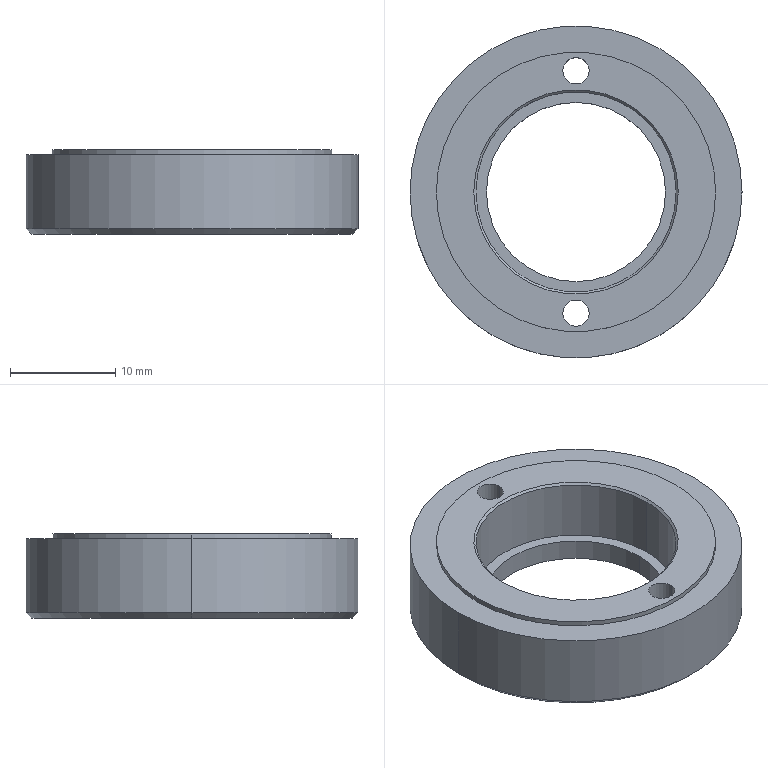Part | SolidWorks | features Chamfer 2, ICE 2, Extrusion 1, HoleWzd 1, MirrorPattern 1 | 1 solid | 20 faces | box 31.5 x 31.5 x 8 mm | volume 3885 mm3 | cylinder 12 | cone 4 | plane 4 | commonest cylinder face diameters 2.5 x4 17 x2 19 x2 26.5 x2 31.5 x2
STEP:
#1=CARTESIAN_POINT('',(-15.25,0.,-4.));
#2=VERTEX_POINT('',#1);
#3=CARTESIAN_POINT('',(15.25,0.,-4.));
#4=VERTEX_POINT('',#3);
#5=CARTESIAN_POINT('',(0.,0.,-4.));
#6=DIRECTION('',(0.,0.,-1.));
#7=DIRECTION('',(1.,0.,0.));
#8=AXIS2_PLACEMENT_3D('',#5,#6,#7);
#9=CIRCLE('',#8,15.25);
#10=EDGE_CURVE('',#2,#4,#9,.T.);
#11=ORIENTED_EDGE('',*,*,#10,.F.);
#12=CARTESIAN_POINT('',(-15.75,0.,-3.5));
#13=VERTEX_POINT('',#12);
#14=CARTESIAN_POINT('',(-15.75,0.,-3.5));
#15=DIRECTION('',(-0.7071,0.,0.7071));
#16=VECTOR('',#15,1000.);
#17=LINE('',#14,#16);
#18=EDGE_CURVE('',#2,#13,#17,.T.);
#19=ORIENTED_EDGE('',*,*,#18,.T.);
#20=CARTESIAN_POINT('',(15.75,0.,-3.5));
#21=VERTEX_POINT('',#20);
#22=CARTESIAN_POINT('',(0.,0.,-3.5));
#23=DIRECTION('',(0.,0.,1.));
#24=DIRECTION('',(1.,0.,0.));
#25=AXIS2_PLACEMENT_3D('',#22,#23,#24);
#26=CIRCLE('',#25,15.75);
#27=EDGE_CURVE('',#21,#13,#26,.T.);
#28=ORIENTED_EDGE('',*,*,#27,.F.);
#29=CARTESIAN_POINT('',(15.75,0.,-3.5));
#30=DIRECTION('',(0.7071,0.,0.7071));
#31=VECTOR('',#30,1000.);
#32=LINE('',#29,#31);
#33=EDGE_CURVE('',#4,#21,#32,.T.);
#34=ORIENTED_EDGE('',*,*,#33,.F.);
#35=EDGE_LOOP('',(#11,#19,#28,#34));
#36=FACE_OUTER_BOUND('',#35,.T.);
#37=CARTESIAN_POINT('',(0.,0.,-3.5));
#38=DIRECTION('',(0.,0.,1.));
#39=DIRECTION('',(1.,0.,0.));
#40=AXIS2_PLACEMENT_3D('',#37,#38,#39);
#41=CONICAL_SURFACE('',#40,15.75,0.7854);
#42=ADVANCED_FACE('',(#36),#41,.T.);
#43=CARTESIAN_POINT('',(13.25,0.,3.55));
#44=VERTEX_POINT('',#43);
#45=CARTESIAN_POINT('',(-13.25,0.,3.55));
#46=VERTEX_POINT('',#45);
#47=CARTESIAN_POINT('',(0.,0.,3.55));
#48=DIRECTION('',(0.,0.,1.));
#49=DIRECTION('',(1.,0.,0.));
#50=AXIS2_PLACEMENT_3D('',#47,#48,#49);
#51=CIRCLE('',#50,13.25);
#52=EDGE_CURVE('',#44,#46,#51,.T.);
#53=ORIENTED_EDGE('',*,*,#52,.T.);
#54=CARTESIAN_POINT('',(-13.25,0.,4.));
#55=VERTEX_POINT('',#54);
#56=CARTESIAN_POINT('',(-13.25,0.,3.55));
#57=DIRECTION('',(0.,0.,1.));
#58=VECTOR('',#57,1000.);
#59=LINE('',#56,#58);
#60=EDGE_CURVE('',#46,#55,#59,.T.);
#61=ORIENTED_EDGE('',*,*,#60,.T.);
#62=CARTESIAN_POINT('',(13.25,0.,4.));
#63=VERTEX_POINT('',#62);
#64=CARTESIAN_POINT('',(0.,0.,4.));
#65=DIRECTION('',(0.,0.,1.));
#66=DIRECTION('',(1.,0.,0.));
#67=AXIS2_PLACEMENT_3D('',#64,#65,#66);
#68=CIRCLE('',#67,13.25);
#69=EDGE_CURVE('',#63,#55,#68,.T.);
#70=ORIENTED_EDGE('',*,*,#69,.F.);
#71=CARTESIAN_POINT('',(13.25,0.,3.55));
#72=DIRECTION('',(0.,0.,1.));
#73=VECTOR('',#72,1000.);
#74=LINE('',#71,#73);
#75=EDGE_CURVE('',#44,#63,#74,.T.);
#76=ORIENTED_EDGE('',*,*,#75,.F.);
#77=EDGE_LOOP('',(#53,#61,#70,#76));
#78=FACE_OUTER_BOUND('',#77,.T.);
#79=CARTESIAN_POINT('',(0.,0.,3.55));
#80=DIRECTION('',(0.,0.,1.));
#81=DIRECTION('',(1.,0.,0.));
#82=AXIS2_PLACEMENT_3D('',#79,#80,#81);
#83=CYLINDRICAL_SURFACE('',#82,13.25);
#84=ADVANCED_FACE('',(#78),#83,.T.);
#85=CARTESIAN_POINT('',(-9.5,0.,3.8));
#86=VERTEX_POINT('',#85);
#87=CARTESIAN_POINT('',(9.5,0.,3.8));
#88=VERTEX_POINT('',#87);
#89=CARTESIAN_POINT('',(0.,0.,3.8));
#90=DIRECTION('',(0.,0.,1.));
#91=DIRECTION('',(1.,0.,0.));
#92=AXIS2_PLACEMENT_3D('',#89,#90,#91);
#93=CIRCLE('',#92,9.5);
#94=EDGE_CURVE('',#86,#88,#93,.T.);
#95=ORIENTED_EDGE('',*,*,#94,.F.);
#96=CARTESIAN_POINT('',(-9.7,0.,4.));
#97=VERTEX_POINT('',#96);
#98=CARTESIAN_POINT('',(-9.5,0.,3.8));
#99=DIRECTION('',(-0.7071,0.,0.7071));
#100=VECTOR('',#99,1000.);
#101=LINE('',#98,#100);
#102=EDGE_CURVE('',#86,#97,#101,.T.);
#103=ORIENTED_EDGE('',*,*,#102,.T.);
#104=CARTESIAN_POINT('',(9.7,0.,4.));
#105=VERTEX_POINT('',#104);
#106=CARTESIAN_POINT('',(0.,0.,4.));
#107=DIRECTION('',(0.,0.,-1.));
#108=DIRECTION('',(1.,0.,0.));
#109=AXIS2_PLACEMENT_3D('',#106,#107,#108);
#110=CIRCLE('',#109,9.7);
#111=EDGE_CURVE('',#105,#97,#110,.T.);
#112=ORIENTED_EDGE('',*,*,#111,.F.);
#113=CARTESIAN_POINT('',(9.5,0.,3.8));
#114=DIRECTION('',(0.7071,0.,0.7071));
#115=VECTOR('',#114,1000.);
#116=LINE('',#113,#115);
#117=EDGE_CURVE('',#88,#105,#116,.T.);
#118=ORIENTED_EDGE('',*,*,#117,.F.);
#119=EDGE_LOOP('',(#95,#103,#112,#118));
#120=FACE_OUTER_BOUND('',#119,.T.);
#121=CARTESIAN_POINT('',(0.,0.,3.8));
#122=DIRECTION('',(0.,0.,1.));
#123=DIRECTION('',(1.,0.,0.));
#124=AXIS2_PLACEMENT_3D('',#121,#122,#123);
#125=CONICAL_SURFACE('',#124,9.5,0.7854);
#126=ADVANCED_FACE('',(#120),#125,.F.);
#127=CARTESIAN_POINT('',(-1.25,11.5,-4.));
#128=VERTEX_POINT('',#127);
#129=CARTESIAN_POINT('',(1.25,11.5,-4.));
#130=VERTEX_POINT('',#129);
#131=CARTESIAN_POINT('',(0.,11.5,-4.));
#132=DIRECTION('',(0.,0.,1.));
#133=DIRECTION('',(1.,0.,0.));
#134=AXIS2_PLACEMENT_3D('',#131,#132,#133);
#135=CIRCLE('',#134,1.25);
#136=EDGE_CURVE('',#128,#130,#135,.T.);
#137=ORIENTED_EDGE('',*,*,#136,.F.);
#138=CARTESIAN_POINT('',(-1.25,11.5,4.));
#139=VERTEX_POINT('',#138);
#140=CARTESIAN_POINT('',(-1.25,11.5,4.));
#141=DIRECTION('',(0.,0.,1.));
#142=VECTOR('',#141,1000.);
#143=LINE('',#140,#142);
#144=EDGE_CURVE('',#128,#139,#143,.T.);
#145=ORIENTED_EDGE('',*,*,#144,.T.);
#146=CARTESIAN_POINT('',(1.25,11.5,4.));
#147=VERTEX_POINT('',#146);
#148=CARTESIAN_POINT('',(0.,11.5,4.));
#149=DIRECTION('',(0.,0.,1.));
#150=DIRECTION('',(1.,0.,0.));
#151=AXIS2_PLACEMENT_3D('',#148,#149,#150);
#152=CIRCLE('',#151,1.25);
#153=EDGE_CURVE('',#139,#147,#152,.T.);
#154=ORIENTED_EDGE('',*,*,#153,.T.);
#155=CARTESIAN_POINT('',(1.25,11.5,4.));
#156=DIRECTION('',(0.,0.,1.));
#157=VECTOR('',#156,1000.);
#158=LINE('',#155,#157);
#159=EDGE_CURVE('',#130,#147,#158,.T.);
#160=ORIENTED_EDGE('',*,*,#159,.F.);
#161=EDGE_LOOP('',(#137,#145,#154,#160));
#162=FACE_OUTER_BOUND('',#161,.T.);
#163=CARTESIAN_POINT('',(0.,11.5,4.));
#164=DIRECTION('',(0.,0.,1.));
#165=DIRECTION('',(1.,0.,0.));
#166=AXIS2_PLACEMENT_3D('',#163,#164,#165);
#167=CYLINDRICAL_SURFACE('',#166,1.25);
#168=ADVANCED_FACE('',(#162),#167,.F.);
#169=CARTESIAN_POINT('',(-1.25,-11.5,-4.));
#170=VERTEX_POINT('',#169);
#171=CARTESIAN_POINT('',(1.25,-11.5,-4.));
#172=VERTEX_POINT('',#171);
#173=CARTESIAN_POINT('',(0.,-11.5,-4.));
#174=DIRECTION('',(0.,0.,1.));
#175=DIRECTION('',(1.,0.,0.));
#176=AXIS2_PLACEMENT_3D('',#173,#174,#175);
#177=CIRCLE('',#176,1.25);
#178=EDGE_CURVE('',#170,#172,#177,.T.);
#179=ORIENTED_EDGE('',*,*,#178,.F.);
#180=CARTESIAN_POINT('',(-1.25,-11.5,4.));
#181=VERTEX_POINT('',#180);
#182=CARTESIAN_POINT('',(-1.25,-11.5,4.));
#183=DIRECTION('',(0.,0.,1.));
#184=VECTOR('',#183,1000.);
#185=LINE('',#182,#184);
#186=EDGE_CURVE('',#170,#181,#185,.T.);
#187=ORIENTED_EDGE('',*,*,#186,.T.);
#188=CARTESIAN_POINT('',(1.25,-11.5,4.));
#189=VERTEX_POINT('',#188);
#190=CARTESIAN_POINT('',(0.,-11.5,4.));
#191=DIRECTION('',(0.,0.,1.));
#192=DIRECTION('',(1.,0.,0.));
#193=AXIS2_PLACEMENT_3D('',#190,#191,#192);
#194=CIRCLE('',#193,1.25);
#195=EDGE_CURVE('',#181,#189,#194,.T.);
#196=ORIENTED_EDGE('',*,*,#195,.T.);
#197=CARTESIAN_POINT('',(1.25,-11.5,4.));
#198=DIRECTION('',(0.,0.,1.));
#199=VECTOR('',#198,1000.);
#200=LINE('',#197,#199);
#201=EDGE_CURVE('',#172,#189,#200,.T.);
#202=ORIENTED_EDGE('',*,*,#201,.F.);
#203=EDGE_LOOP('',(#179,#187,#196,#202));
#204=FACE_OUTER_BOUND('',#203,.T.);
#205=CARTESIAN_POINT('',(0.,-11.5,4.));
#206=DIRECTION('',(0.,0.,1.));
#207=DIRECTION('',(1.,0.,0.));
#208=AXIS2_PLACEMENT_3D('',#205,#206,#207);
#209=CYLINDRICAL_SURFACE('',#208,1.25);
#210=ADVANCED_FACE('',(#204),#209,.F.);
#211=CARTESIAN_POINT('',(8.5,0.,-2.));
#212=VERTEX_POINT('',#211);
#213=CARTESIAN_POINT('',(-8.5,0.,-2.));
#214=VERTEX_POINT('',#213);
#215=CARTESIAN_POINT('',(0.,0.,-2.));
#216=DIRECTION('',(0.,0.,-1.));
#217=DIRECTION('',(-1.,0.,0.));
#218=AXIS2_PLACEMENT_3D('',#215,#216,#217);
#219=CIRCLE('',#218,8.5);
#220=EDGE_CURVE('',#212,#214,#219,.T.);
#221=ORIENTED_EDGE('',*,*,#220,.F.);
#222=CARTESIAN_POINT('',(8.5,0.,-4.));
#223=VERTEX_POINT('',#222);
#224=CARTESIAN_POINT('',(8.5,0.,-2.));
#225=DIRECTION('',(0.,0.,-1.));
#226=VECTOR('',#225,1000.);
#227=LINE('',#224,#226);
#228=EDGE_CURVE('',#212,#223,#227,.T.);
#229=ORIENTED_EDGE('',*,*,#228,.T.);
#230=CARTESIAN_POINT('',(-8.5,0.,-4.));
#231=VERTEX_POINT('',#230);
#232=CARTESIAN_POINT('',(0.,0.,-4.));
#233=DIRECTION('',(0.,0.,-1.));
#234=DIRECTION('',(-1.,0.,0.));
#235=AXIS2_PLACEMENT_3D('',#232,#233,#234);
#236=CIRCLE('',#235,8.5);
#237=EDGE_CURVE('',#223,#231,#236,.T.);
#238=ORIENTED_EDGE('',*,*,#237,.T.);
#239=CARTESIAN_POINT('',(-8.5,0.,-2.));
#240=DIRECTION('',(0.,0.,-1.));
#241=VECTOR('',#240,1000.);
#242=LINE('',#239,#241);
#243=EDGE_CURVE('',#214,#231,#242,.T.);
#244=ORIENTED_EDGE('',*,*,#243,.F.);
#245=EDGE_LOOP('',(#221,#229,#238,#244));
#246=FACE_OUTER_BOUND('',#245,.T.);
#247=CARTESIAN_POINT('',(0.,0.,-2.));
#248=DIRECTION('',(0.,0.,-1.));
#249=DIRECTION('',(-1.,0.,0.));
#250=AXIS2_PLACEMENT_3D('',#247,#248,#249);
#251=CYLINDRICAL_SURFACE('',#250,8.5);
#252=ADVANCED_FACE('',(#246),#251,.F.);
#253=ORIENTED_EDGE('',*,*,#94,.T.);
#254=CARTESIAN_POINT('',(9.5,0.,-2.));
#255=VERTEX_POINT('',#254);
#256=CARTESIAN_POINT('',(9.5,0.,4.));
#257=DIRECTION('',(0.,0.,-1.));
#258=VECTOR('',#257,1000.);
#259=LINE('',#256,#258);
#260=EDGE_CURVE('',#88,#255,#259,.T.);
#261=ORIENTED_EDGE('',*,*,#260,.T.);
#262=CARTESIAN_POINT('',(-9.5,0.,-2.));
#263=VERTEX_POINT('',#262);
#264=CARTESIAN_POINT('',(0.,0.,-2.));
#265=DIRECTION('',(0.,0.,-1.));
#266=DIRECTION('',(-1.,0.,0.));
#267=AXIS2_PLACEMENT_3D('',#264,#265,#266);
#268=CIRCLE('',#267,9.5);
#269=EDGE_CURVE('',#255,#263,#268,.T.);
#270=ORIENTED_EDGE('',*,*,#269,.T.);
#271=CARTESIAN_POINT('',(-9.5,0.,4.));
#272=DIRECTION('',(0.,0.,-1.));
#273=VECTOR('',#272,1000.);
#274=LINE('',#271,#273);
#275=EDGE_CURVE('',#86,#263,#274,.T.);
#276=ORIENTED_EDGE('',*,*,#275,.F.);
#277=EDGE_LOOP('',(#253,#261,#270,#276));
#278=FACE_OUTER_BOUND('',#277,.T.);
#279=CARTESIAN_POINT('',(0.,0.,4.));
#280=DIRECTION('',(0.,0.,-1.));
#281=DIRECTION('',(-1.,0.,0.));
#282=AXIS2_PLACEMENT_3D('',#279,#280,#281);
#283=CYLINDRICAL_SURFACE('',#282,9.5);
#284=ADVANCED_FACE('',(#278),#283,.F.);
#285=CARTESIAN_POINT('',(15.75,0.,3.55));
#286=VERTEX_POINT('',#285);
#287=CARTESIAN_POINT('',(-15.75,0.,3.55));
#288=VERTEX_POINT('',#287);
#289=CARTESIAN_POINT('',(0.,0.,3.55));
#290=DIRECTION('',(0.,0.,1.));
#291=DIRECTION('',(1.,0.,0.));
#292=AXIS2_PLACEMENT_3D('',#289,#290,#291);
#293=CIRCLE('',#292,15.75);
#294=EDGE_CURVE('',#286,#288,#293,.T.);
#295=ORIENTED_EDGE('',*,*,#294,.F.);
#296=CARTESIAN_POINT('',(15.75,0.,4.));
#297=DIRECTION('',(0.,0.,-1.));
#298=VECTOR('',#297,1000.);
#299=LINE('',#296,#298);
#300=EDGE_CURVE('',#286,#21,#299,.T.);
#301=ORIENTED_EDGE('',*,*,#300,.T.);
#302=ORIENTED_EDGE('',*,*,#27,.T.);
#303=CARTESIAN_POINT('',(-15.75,0.,4.));
#304=DIRECTION('',(0.,0.,-1.));
#305=VECTOR('',#304,1000.);
#306=LINE('',#303,#305);
#307=EDGE_CURVE('',#288,#13,#306,.T.);
#308=ORIENTED_EDGE('',*,*,#307,.F.);
#309=EDGE_LOOP('',(#295,#301,#302,#308));
#310=FACE_OUTER_BOUND('',#309,.T.);
#311=CARTESIAN_POINT('',(0.,0.,4.));
#312=DIRECTION('',(0.,0.,-1.));
#313=DIRECTION('',(-1.,0.,0.));
#314=AXIS2_PLACEMENT_3D('',#311,#312,#313);
#315=CYLINDRICAL_SURFACE('',#314,15.75);
#316=ADVANCED_FACE('',(#310),#315,.T.);
#317=CARTESIAN_POINT('',(0.,-11.5,4.));
#318=DIRECTION('',(0.,0.,1.));
#319=DIRECTION('',(1.,0.,0.));
#320=AXIS2_PLACEMENT_3D('',#317,#318,#319);
#321=CIRCLE('',#320,1.25);
#322=EDGE_CURVE('',#189,#181,#321,.T.);
#323=ORIENTED_EDGE('',*,*,#322,.F.);
#324=ORIENTED_EDGE('',*,*,#195,.F.);
#325=EDGE_LOOP('',(#323,#324));
#326=FACE_BOUND('',#325,.T.);
#327=CARTESIAN_POINT('',(0.,11.5,4.));
#328=DIRECTION('',(0.,0.,1.));
#329=DIRECTION('',(1.,0.,0.));
#330=AXIS2_PLACEMENT_3D('',#327,#328,#329);
#331=CIRCLE('',#330,1.25);
#332=EDGE_CURVE('',#147,#139,#331,.T.);
#333=ORIENTED_EDGE('',*,*,#332,.F.);
#334=ORIENTED_EDGE('',*,*,#153,.F.);
#335=EDGE_LOOP('',(#333,#334));
#336=FACE_BOUND('',#335,.T.);
#337=ORIENTED_EDGE('',*,*,#111,.T.);
#338=CARTESIAN_POINT('',(0.,0.,4.));
#339=DIRECTION('',(0.,0.,-1.));
#340=DIRECTION('',(1.,0.,0.));
#341=AXIS2_PLACEMENT_3D('',#338,#339,#340);
#342=CIRCLE('',#341,9.7);
#343=EDGE_CURVE('',#97,#105,#342,.T.);
#344=ORIENTED_EDGE('',*,*,#343,.T.);
#345=EDGE_LOOP('',(#337,#344));
#346=FACE_BOUND('',#345,.T.);
#347=ORIENTED_EDGE('',*,*,#69,.T.);
#348=CARTESIAN_POINT('',(0.,0.,4.));
#349=DIRECTION('',(0.,0.,1.));
#350=DIRECTION('',(1.,0.,0.));
#351=AXIS2_PLACEMENT_3D('',#348,#349,#350);
#352=CIRCLE('',#351,13.25);
#353=EDGE_CURVE('',#55,#63,#352,.T.);
#354=ORIENTED_EDGE('',*,*,#353,.T.);
#355=EDGE_LOOP('',(#347,#354));
#356=FACE_OUTER_BOUND('',#355,.T.);
#357=CARTESIAN_POINT('',(0.,0.,4.));
#358=DIRECTION('',(0.,0.,1.));
#359=DIRECTION('',(1.,0.,0.));
#360=AXIS2_PLACEMENT_3D('',#357,#358,#359);
#361=PLANE('',#360);
#362=ADVANCED_FACE('',(#326,#336,#346,#356),#361,.T.);
#363=ORIENTED_EDGE('',*,*,#300,.F.);
#364=CARTESIAN_POINT('',(0.,0.,3.55));
#365=DIRECTION('',(0.,0.,1.));
#366=DIRECTION('',(1.,0.,0.));
#367=AXIS2_PLACEMENT_3D('',#364,#365,#366);
#368=CIRCLE('',#367,15.75);
#369=EDGE_CURVE('',#288,#286,#368,.T.);
#370=ORIENTED_EDGE('',*,*,#369,.F.);
#371=ORIENTED_EDGE('',*,*,#307,.T.);
#372=CARTESIAN_POINT('',(0.,0.,-3.5));
#373=DIRECTION('',(0.,0.,1.));
#374=DIRECTION('',(1.,0.,0.));
#375=AXIS2_PLACEMENT_3D('',#372,#373,#374);
#376=CIRCLE('',#375,15.75);
#377=EDGE_CURVE('',#13,#21,#376,.T.);
#378=ORIENTED_EDGE('',*,*,#377,.T.);
#379=EDGE_LOOP('',(#363,#370,#371,#378));
#380=FACE_OUTER_BOUND('',#379,.T.);
#381=CARTESIAN_POINT('',(0.,0.,4.));
#382=DIRECTION('',(0.,0.,-1.));
#383=DIRECTION('',(-1.,0.,0.));
#384=AXIS2_PLACEMENT_3D('',#381,#382,#383);
#385=CYLINDRICAL_SURFACE('',#384,15.75);
#386=ADVANCED_FACE('',(#380),#385,.T.);
#387=ORIENTED_EDGE('',*,*,#260,.F.);
#388=CARTESIAN_POINT('',(0.,0.,3.8));
#389=DIRECTION('',(0.,0.,1.));
#390=DIRECTION('',(1.,0.,0.));
#391=AXIS2_PLACEMENT_3D('',#388,#389,#390);
#392=CIRCLE('',#391,9.5);
#393=EDGE_CURVE('',#88,#86,#392,.T.);
#394=ORIENTED_EDGE('',*,*,#393,.T.);
#395=ORIENTED_EDGE('',*,*,#275,.T.);
#396=CARTESIAN_POINT('',(0.,0.,-2.));
#397=DIRECTION('',(0.,0.,-1.));
#398=DIRECTION('',(-1.,0.,0.));
#399=AXIS2_PLACEMENT_3D('',#396,#397,#398);
#400=CIRCLE('',#399,9.5);
#401=EDGE_CURVE('',#263,#255,#400,.T.);
#402=ORIENTED_EDGE('',*,*,#401,.T.);
#403=EDGE_LOOP('',(#387,#394,#395,#402));
#404=FACE_OUTER_BOUND('',#403,.T.);
#405=CARTESIAN_POINT('',(0.,0.,4.));
#406=DIRECTION('',(0.,0.,-1.));
#407=DIRECTION('',(-1.,0.,0.));
#408=AXIS2_PLACEMENT_3D('',#405,#406,#407);
#409=CYLINDRICAL_SURFACE('',#408,9.5);
#410=ADVANCED_FACE('',(#404),#409,.F.);
#411=CARTESIAN_POINT('',(0.,0.,-4.));
#412=DIRECTION('',(0.,0.,-1.));
#413=DIRECTION('',(1.,0.,0.));
#414=AXIS2_PLACEMENT_3D('',#411,#412,#413);
#415=CIRCLE('',#414,15.25);
#416=EDGE_CURVE('',#4,#2,#415,.T.);
#417=ORIENTED_EDGE('',*,*,#416,.T.);
#418=ORIENTED_EDGE('',*,*,#10,.T.);
#419=EDGE_LOOP('',(#417,#418));
#420=FACE_OUTER_BOUND('',#419,.T.);
#421=CARTESIAN_POINT('',(0.,11.5,-4.));
#422=DIRECTION('',(0.,0.,1.));
#423=DIRECTION('',(1.,0.,0.));
#424=AXIS2_PLACEMENT_3D('',#421,#422,#423);
#425=CIRCLE('',#424,1.25);
#426=EDGE_CURVE('',#130,#128,#425,.T.);
#427=ORIENTED_EDGE('',*,*,#426,.T.);
#428=ORIENTED_EDGE('',*,*,#136,.T.);
#429=EDGE_LOOP('',(#427,#428));
#430=FACE_BOUND('',#429,.T.);
#431=CARTESIAN_POINT('',(0.,-11.5,-4.));
#432=DIRECTION('',(0.,0.,1.));
#433=DIRECTION('',(1.,0.,0.));
#434=AXIS2_PLACEMENT_3D('',#431,#432,#433);
#435=CIRCLE('',#434,1.25);
#436=EDGE_CURVE('',#172,#170,#435,.T.);
#437=ORIENTED_EDGE('',*,*,#436,.T.);
#438=ORIENTED_EDGE('',*,*,#178,.T.);
#439=EDGE_LOOP('',(#437,#438));
#440=FACE_BOUND('',#439,.T.);
#441=CARTESIAN_POINT('',(0.,0.,-4.));
#442=DIRECTION('',(0.,0.,-1.));
#443=DIRECTION('',(-1.,0.,0.));
#444=AXIS2_PLACEMENT_3D('',#441,#442,#443);
#445=CIRCLE('',#444,8.5);
#446=EDGE_CURVE('',#231,#223,#445,.T.);
#447=ORIENTED_EDGE('',*,*,#446,.F.);
#448=ORIENTED_EDGE('',*,*,#237,.F.);
#449=EDGE_LOOP('',(#447,#448));
#450=FACE_BOUND('',#449,.T.);
#451=CARTESIAN_POINT('',(0.,0.,-4.));
#452=DIRECTION('',(0.,0.,1.));
#453=DIRECTION('',(1.,0.,0.));
#454=AXIS2_PLACEMENT_3D('',#451,#452,#453);
#455=PLANE('',#454);
#456=ADVANCED_FACE('',(#420,#430,#440,#450),#455,.F.);
#457=CARTESIAN_POINT('',(0.,0.,-2.));
#458=DIRECTION('',(0.,0.,-1.));
#459=DIRECTION('',(-1.,0.,0.));
#460=AXIS2_PLACEMENT_3D('',#457,#458,#459);
#461=CIRCLE('',#460,8.5);
#462=EDGE_CURVE('',#214,#212,#461,.T.);
#463=ORIENTED_EDGE('',*,*,#462,.T.);
#464=ORIENTED_EDGE('',*,*,#220,.T.);
#465=EDGE_LOOP('',(#463,#464));
#466=FACE_BOUND('',#465,.T.);
#467=ORIENTED_EDGE('',*,*,#401,.F.);
#468=ORIENTED_EDGE('',*,*,#269,.F.);
#469=EDGE_LOOP('',(#467,#468));
#470=FACE_OUTER_BOUND('',#469,.T.);
#471=CARTESIAN_POINT('',(0.,0.,-2.));
#472=DIRECTION('',(0.,0.,-1.));
#473=DIRECTION('',(-1.,0.,0.));
#474=AXIS2_PLACEMENT_3D('',#471,#472,#473);
#475=PLANE('',#474);
#476=ADVANCED_FACE('',(#466,#470),#475,.F.);
#477=ORIENTED_EDGE('',*,*,#228,.F.);
#478=ORIENTED_EDGE('',*,*,#462,.F.);
#479=ORIENTED_EDGE('',*,*,#243,.T.);
#480=ORIENTED_EDGE('',*,*,#446,.T.);
#481=EDGE_LOOP('',(#477,#478,#479,#480));
#482=FACE_OUTER_BOUND('',#481,.T.);
#483=CARTESIAN_POINT('',(0.,0.,-2.));
#484=DIRECTION('',(0.,0.,-1.));
#485=DIRECTION('',(-1.,0.,0.));
#486=AXIS2_PLACEMENT_3D('',#483,#484,#485);
#487=CYLINDRICAL_SURFACE('',#486,8.5);
#488=ADVANCED_FACE('',(#482),#487,.F.);
#489=ORIENTED_EDGE('',*,*,#186,.F.);
#490=ORIENTED_EDGE('',*,*,#436,.F.);
#491=ORIENTED_EDGE('',*,*,#201,.T.);
#492=ORIENTED_EDGE('',*,*,#322,.T.);
#493=EDGE_LOOP('',(#489,#490,#491,#492));
#494=FACE_OUTER_BOUND('',#493,.T.);
#495=CARTESIAN_POINT('',(0.,-11.5,4.));
#496=DIRECTION('',(0.,0.,1.));
#497=DIRECTION('',(1.,0.,0.));
#498=AXIS2_PLACEMENT_3D('',#495,#496,#497);
#499=CYLINDRICAL_SURFACE('',#498,1.25);
#500=ADVANCED_FACE('',(#494),#499,.F.);
#501=ORIENTED_EDGE('',*,*,#144,.F.);
#502=ORIENTED_EDGE('',*,*,#426,.F.);
#503=ORIENTED_EDGE('',*,*,#159,.T.);
#504=ORIENTED_EDGE('',*,*,#332,.T.);
#505=EDGE_LOOP('',(#501,#502,#503,#504));
#506=FACE_OUTER_BOUND('',#505,.T.);
#507=CARTESIAN_POINT('',(0.,11.5,4.));
#508=DIRECTION('',(0.,0.,1.));
#509=DIRECTION('',(1.,0.,0.));
#510=AXIS2_PLACEMENT_3D('',#507,#508,#509);
#511=CYLINDRICAL_SURFACE('',#510,1.25);
#512=ADVANCED_FACE('',(#506),#511,.F.);
#513=ORIENTED_EDGE('',*,*,#102,.F.);
#514=ORIENTED_EDGE('',*,*,#393,.F.);
#515=ORIENTED_EDGE('',*,*,#117,.T.);
#516=ORIENTED_EDGE('',*,*,#343,.F.);
#517=EDGE_LOOP('',(#513,#514,#515,#516));
#518=FACE_OUTER_BOUND('',#517,.T.);
#519=CARTESIAN_POINT('',(0.,0.,3.8));
#520=DIRECTION('',(0.,0.,1.));
#521=DIRECTION('',(1.,0.,0.));
#522=AXIS2_PLACEMENT_3D('',#519,#520,#521);
#523=CONICAL_SURFACE('',#522,9.5,0.7854);
#524=ADVANCED_FACE('',(#518),#523,.F.);
#525=ORIENTED_EDGE('',*,*,#52,.F.);
#526=CARTESIAN_POINT('',(0.,0.,3.55));
#527=DIRECTION('',(0.,0.,1.));
#528=DIRECTION('',(1.,0.,0.));
#529=AXIS2_PLACEMENT_3D('',#526,#527,#528);
#530=CIRCLE('',#529,13.25);
#531=EDGE_CURVE('',#46,#44,#530,.T.);
#532=ORIENTED_EDGE('',*,*,#531,.F.);
#533=EDGE_LOOP('',(#525,#532));
#534=FACE_BOUND('',#533,.T.);
#535=ORIENTED_EDGE('',*,*,#369,.T.);
#536=ORIENTED_EDGE('',*,*,#294,.T.);
#537=EDGE_LOOP('',(#535,#536));
#538=FACE_OUTER_BOUND('',#537,.T.);
#539=CARTESIAN_POINT('',(0.,0.,3.55));
#540=DIRECTION('',(0.,0.,1.));
#541=DIRECTION('',(1.,0.,0.));
#542=AXIS2_PLACEMENT_3D('',#539,#540,#541);
#543=PLANE('',#542);
#544=ADVANCED_FACE('',(#534,#538),#543,.T.);
#545=ORIENTED_EDGE('',*,*,#60,.F.);
#546=ORIENTED_EDGE('',*,*,#531,.T.);
#547=ORIENTED_EDGE('',*,*,#75,.T.);
#548=ORIENTED_EDGE('',*,*,#353,.F.);
#549=EDGE_LOOP('',(#545,#546,#547,#548));
#550=FACE_OUTER_BOUND('',#549,.T.);
#551=CARTESIAN_POINT('',(0.,0.,3.55));
#552=DIRECTION('',(0.,0.,1.));
#553=DIRECTION('',(1.,0.,0.));
#554=AXIS2_PLACEMENT_3D('',#551,#552,#553);
#555=CYLINDRICAL_SURFACE('',#554,13.25);
#556=ADVANCED_FACE('',(#550),#555,.T.);
#557=ORIENTED_EDGE('',*,*,#18,.F.);
#558=ORIENTED_EDGE('',*,*,#416,.F.);
#559=ORIENTED_EDGE('',*,*,#33,.T.);
#560=ORIENTED_EDGE('',*,*,#377,.F.);
#561=EDGE_LOOP('',(#557,#558,#559,#560));
#562=FACE_OUTER_BOUND('',#561,.T.);
#563=CARTESIAN_POINT('',(0.,0.,-3.5));
#564=DIRECTION('',(0.,0.,1.));
#565=DIRECTION('',(1.,0.,0.));
#566=AXIS2_PLACEMENT_3D('',#563,#564,#565);
#567=CONICAL_SURFACE('',#566,15.75,0.7854);
#568=ADVANCED_FACE('',(#562),#567,.T.);
#569=CLOSED_SHELL('',(#42,#84,#126,#168,#210,#252,#284,#316,#362,#386,#410,#456,#476,#488,#500,#512,#524,#544,#556,#568));
#570=MANIFOLD_SOLID_BREP('',#569);
#571=CARTESIAN_POINT('',(0.,0.,0.));
#572=DIRECTION('',(0.,0.,1.));
#573=DIRECTION('',(1.,0.,0.));
#574=AXIS2_PLACEMENT_3D('',#571,#572,#573);
#575=(LENGTH_UNIT()NAMED_UNIT(*)SI_UNIT(.MILLI.,.METRE.));
#576=UNCERTAINTY_MEASURE_WITH_UNIT(LENGTH_MEASURE(0.00001),#575,'','');
#577=(NAMED_UNIT(*)PLANE_ANGLE_UNIT()SI_UNIT($,.RADIAN.));
#578=(NAMED_UNIT(*)SI_UNIT($,.STERADIAN.)SOLID_ANGLE_UNIT());
#579=(GEOMETRIC_REPRESENTATION_CONTEXT(3)GLOBAL_UNCERTAINTY_ASSIGNED_CONTEXT((#576))GLOBAL_UNIT_ASSIGNED_CONTEXT((#575,#577,#578))REPRESENTATION_CONTEXT('',''));
#580=ADVANCED_BREP_SHAPE_REPRESENTATION('',(#570,#574),#579);